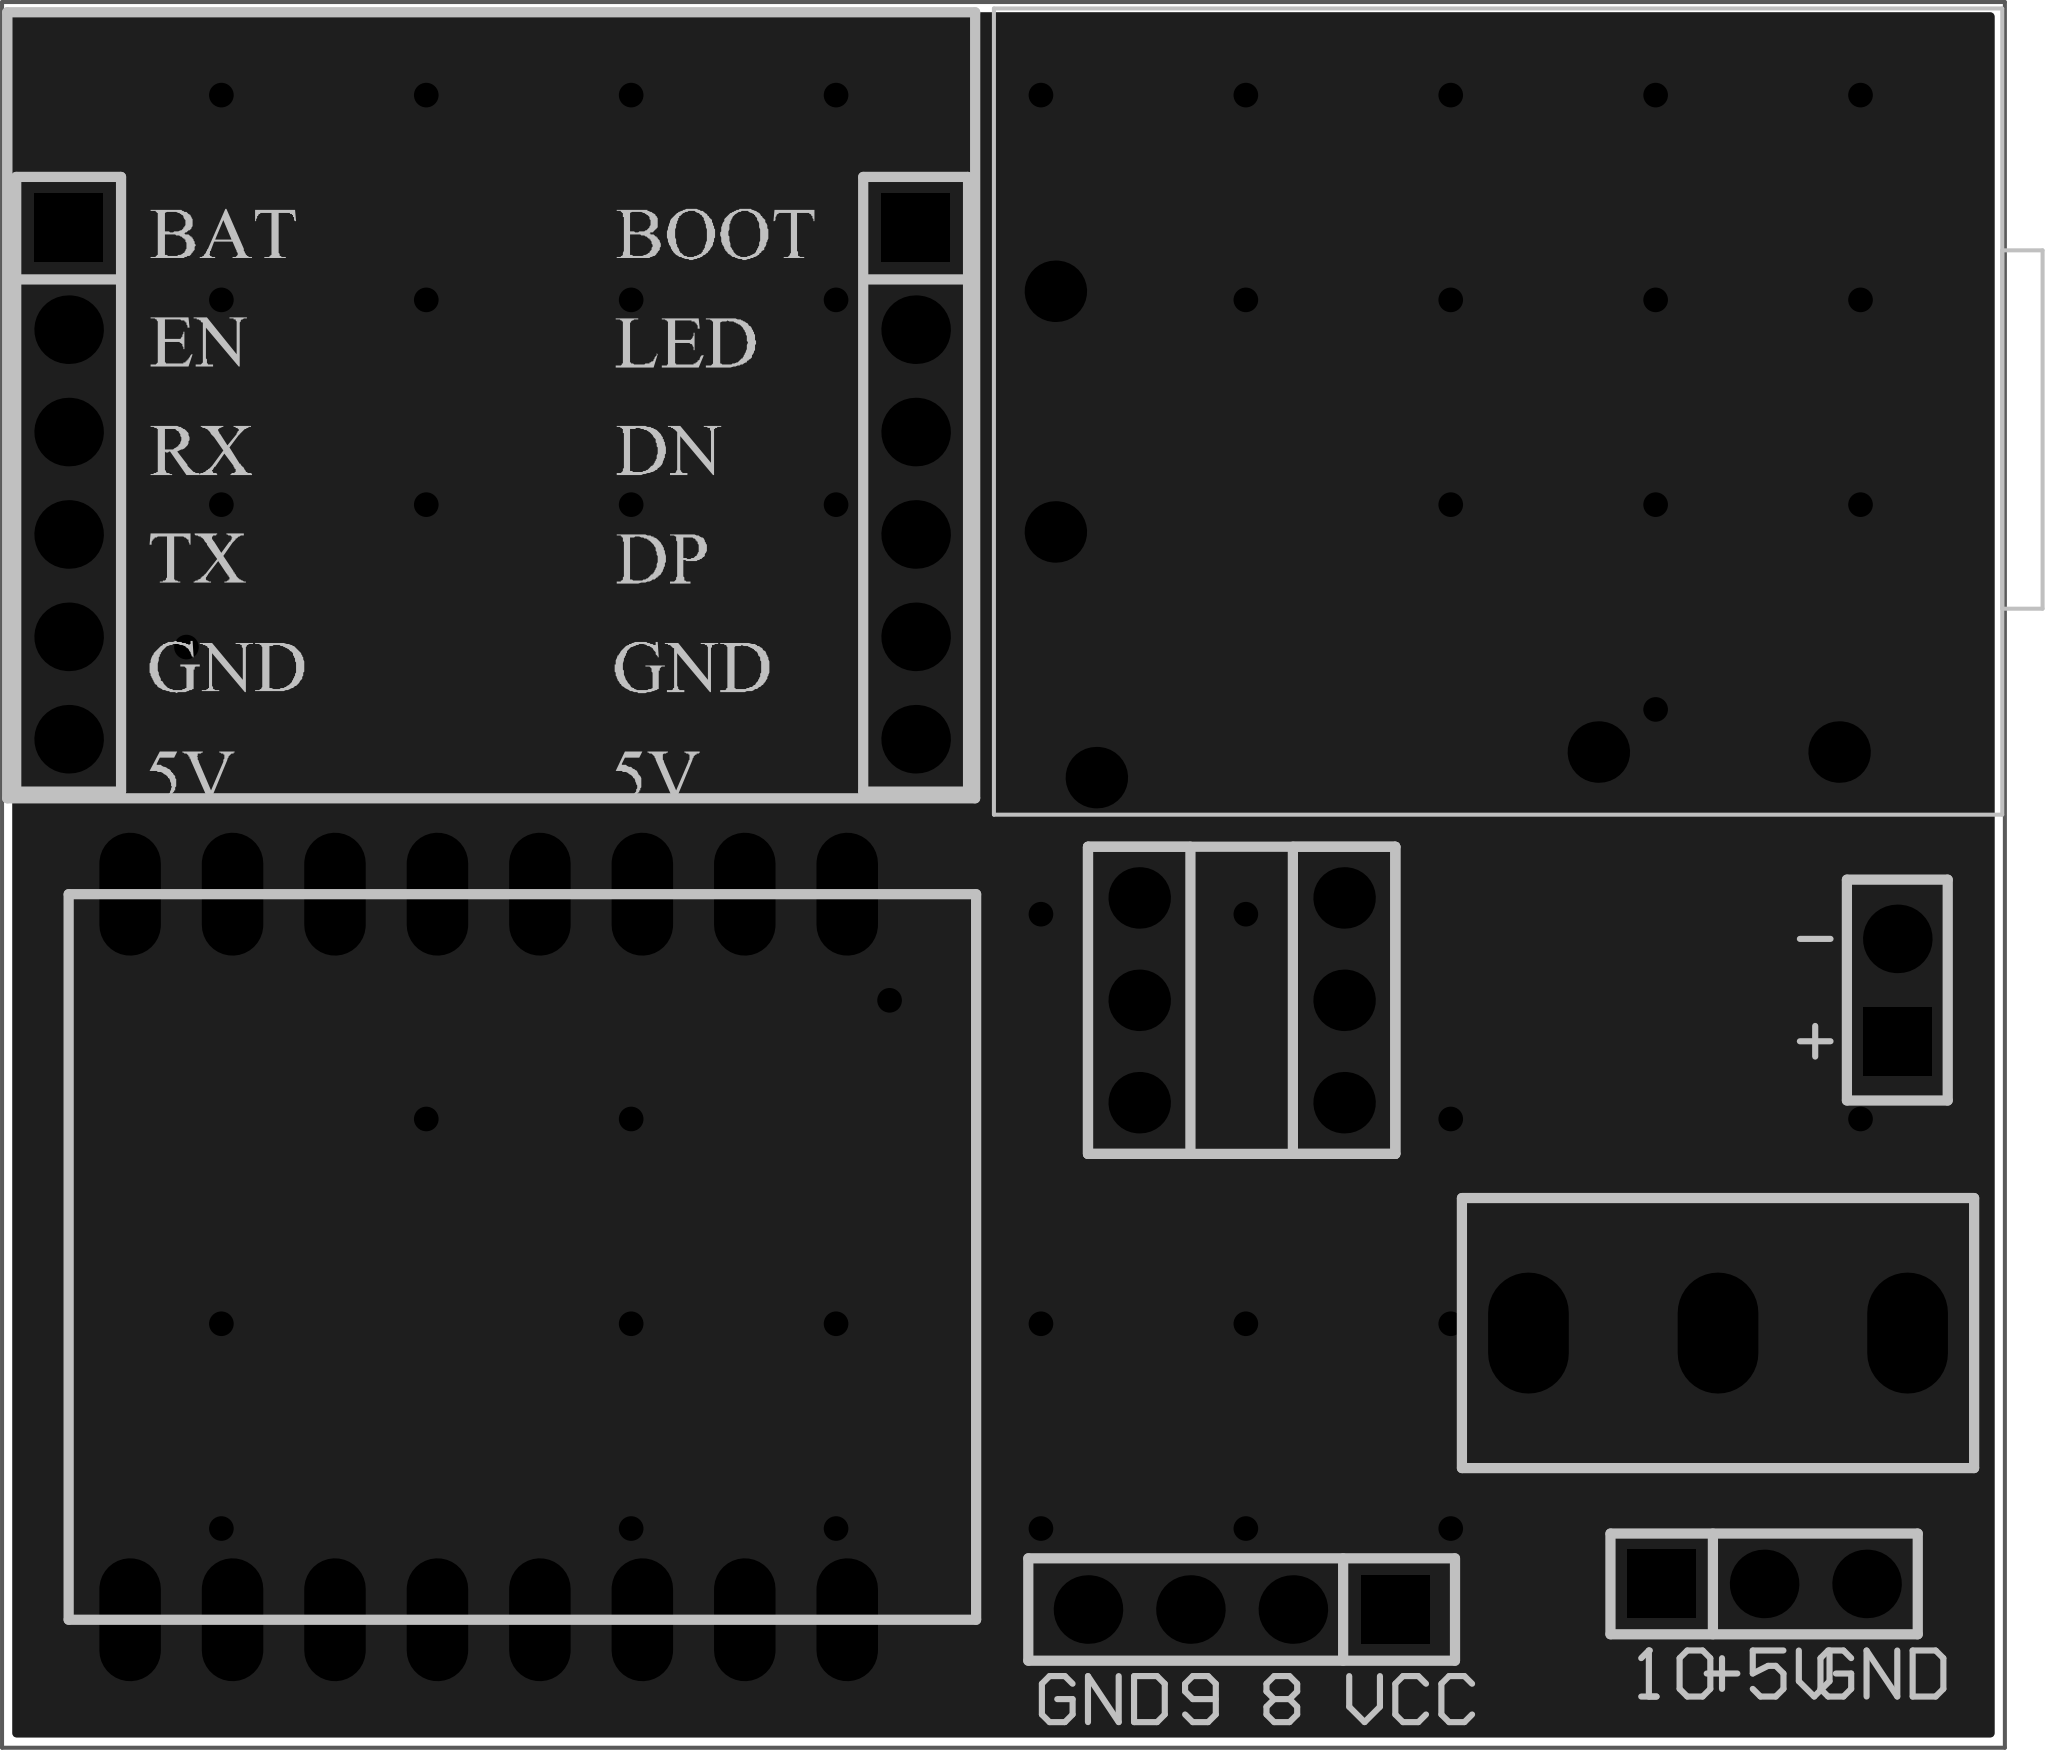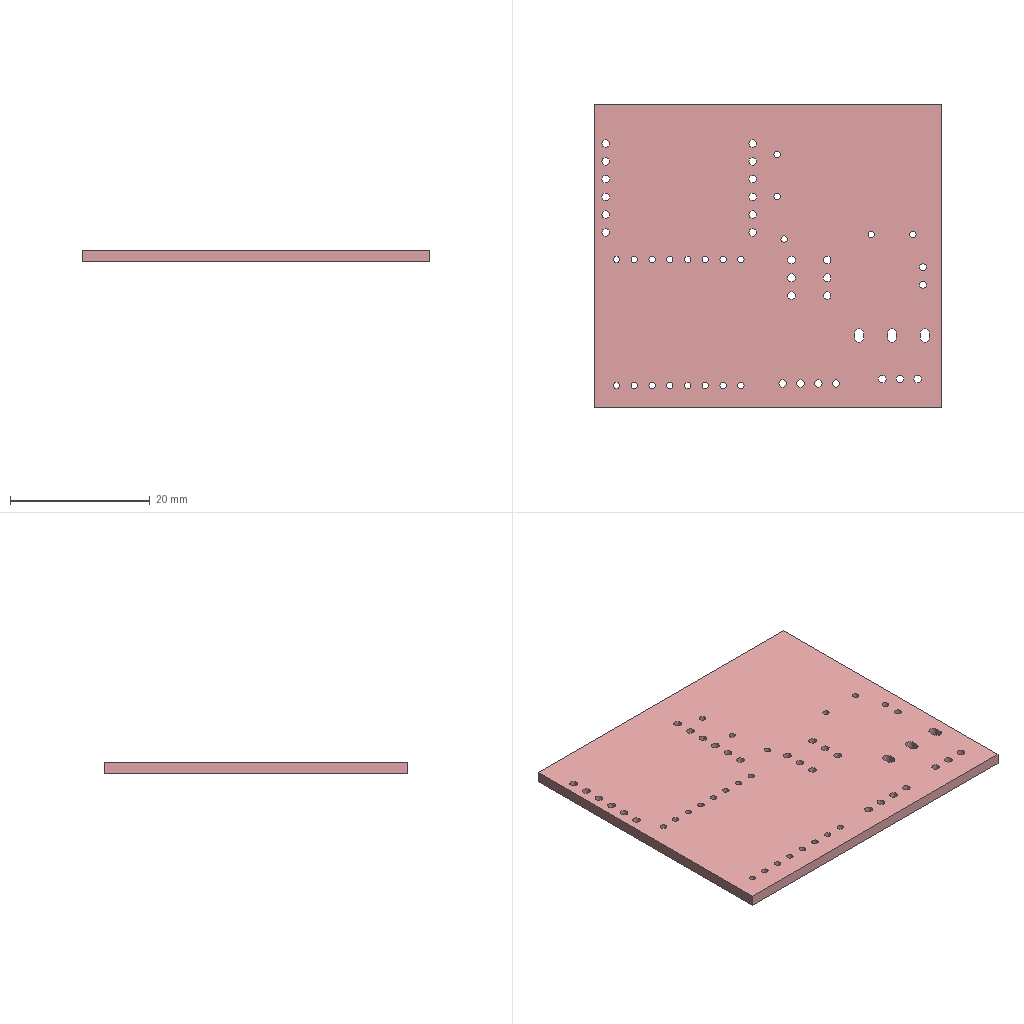Circuit board layout | Altium Designer | box 49.7 x 43.3 x 1.6 mm
Layer stack:
# Altium Designer layer stack of  (unit mm; dielectric type: 0 none, 1 core, 2 prepreg, 3 surface material)
index,name,kind,layer,copper_thickness_mm,dielectric_type,dielectric_thickness_mm,dielectric_material,dielectric_constant
0,Top Paste Mask Layer,other,,,,,,
1,Top Silkscreen Layer,other,,,,,,
2,Top Solder Mask Layer,dielectric,,,3,0.01,,3.3
3,Top Layer,copper,Top Layer,0.035,,,,
4,Dielectric1,dielectric,,,3,1.51,FR4,4.5
5,Bottom Layer,copper,Bottom Layer,0.035,,,,
6,Bottom Solder Mask Layer,dielectric,,,3,0.01,,3.3
7,Bottom Silkscreen Layer,other,,,,,,
8,Bottom Paste Mask Layer,other,,,,,,
# drill layer pairs: low layer,high layer
drill_pair,Top Layer,Bottom Layer
Part placement:
Designator,Comment,Layer,Footprint,Center-X(mm),Center-Y(mm),Rotation
H1,,TopLayer,HDR-TH_3P-P2.54-V-M,161.036,111.506,0
H2,,TopLayer,HDR-TH_2P-P2.54-V-F,164.338,126.238,90
H9,,TopLayer,HDR-TH_4P-P2.54-V-F,148.082,110.871,180
S1,SS-12D10L5,TopLayer,SS-12D10L5,159.893,117.729,0
U3,,TopLayer,【封装Supermini】,129.413,119.617,90
U4,,TopLayer,ML307C-GC核心板,129.499,138.811,0
U5,,TopLayer,5V2A充放电一体模块,153.179,137.541,90
U6,INMP441,TopLayer,INMP441,148.082,125.984,0
Pad and via stacks:
# Altium Designer via and pad stacks of  (unit mm). Each distinct definition once, with the count of objects using it.
# via: kind,start_layer,end_layer,hole_mm,diameter_mm,mode(0 simple;1 top-mid-bottom;2 full stack),diameter_per_layer,count,example_net
# pad: kind,layer,hole_mm,hole_type(0 round;1 square;2 slot),plating,top_size,top_shape(1 round;2 rect;3 octagon;9 rounded rect),mid_size,bottom_size,mode,footprint,size_per_layer,count,example
pad,Multi-Layer,1.1,0,plated,1.7x1.7,2,1.7x1.7,1.7x1.7,0,HDR-TH_3P-P2.54-V-M,,1,H1.1
pad,Multi-Layer,1.1,0,plated,1.7x1.7,1,1.7x1.7,1.7x1.7,0,HDR-TH_3P-P2.54-V-M,,2,H1.2
pad,Multi-Layer,1,0,plated,1.7x1.7,2,1.7x1.7,1.7x1.7,0,HDR-TH_2P-P2.54-V-F,,1,H2.1
pad,Multi-Layer,1,0,plated,1.7x1.7,1,1.7x1.7,1.7x1.7,0,HDR-TH_2P-P2.54-V-F,,1,H2.2
pad,Multi-Layer,1.1,0,plated,1.7x1.7,2,1.7x1.7,1.7x1.7,0,HDR-TH_4P-P2.54-V-F,,1,H9.1
pad,Multi-Layer,1.1,0,plated,1.7x1.7,1,1.7x1.7,1.7x1.7,0,HDR-TH_4P-P2.54-V-F,,3,H9.2
pad,Multi-Layer,1.3,2,plated,2x3,1,2x3,2x3,0,SS-12D10L5,,3,S1.1
pad,Multi-Layer,0.9144,0,plated,1.524x3.048,1,1.524x3.048,1.524x3.048,0,\u00A1\u00BE\u00B7\u00E2\u00D7\u00B0Supermini\u00A1\u00BF,,16,U3.1
pad,Multi-Layer,1.1,0,plated,1.7x1.7,2,1.7x1.7,1.7x1.7,0,ML307C-GC\u00BA\u00CB\u00D0\u00C4\u00B0\u00E5,,2,U4.1
pad,Multi-Layer,1.1,0,plated,1.7x1.7,1,1.7x1.7,1.7x1.7,0,ML307C-GC\u00BA\u00CB\u00D0\u00C4\u00B0\u00E5,,10,U4.2
pad,Multi-Layer,0.9144,0,plated,1.524x1.524,1,1.524x1.524,1.524x1.524,0,5V2A\u00B3\u00E4\u00B7\u00C5\u00B5\u00E7\u00D2\u00BB\u00CC\u00E5\u00C4\u00A3\u00BF\u00E9,,5,U5.3
pad,Multi-Layer,1.1,0,plated,1.524x1.524,1,1.524x1.524,1.524x1.524,0,INMP441,,6,U6.1
via,Top Layer,Bottom Layer,0.3048,0.61,0,,45,VCC
Copper pours:
name,layer,net,type(0 solid;1 hatched;2 none)
Top Layer-GND,Top Layer,GND,0
Bottom Layer-GND,Bottom Layer,GND,0
Design rules, without the lines most boards share:
# Altium Designer design rules of  (exported by Altium Designer, unit mm)
# columns: name | kind | enabled | priority | scope1 | scope2 | descriptor | typed fields (field=value)
Copper_copperRegion_copperThickness1oz | 0 | disabled | 4 | All | All | Clearance Constraint (Gap=5.984mil) (Disabled)(All),(All) | gap=0.152
Copper_copperRegion_copperThickness1oz_1 | 63 | disabled | 4 | All | All | Board Clearance Constraint (Gap=0mil) (Disabled)(All) |
Copper_copperRegion_Copper_copperRegion | 0 | disabled | 5 | All | All | Clearance Constraint (Gap=5.984mil) (Disabled)(All),(All) | gap=0.152
Copper_copperRegion_Copper_copperRegion_1 | 63 | disabled | 5 | All | All | Board Clearance Constraint (Gap=0mil) (Disabled)(All) |
copperThickness1oz | 0 | enabled | 6 | All | All | Clearance Constraint (Gap=5.984mil) (All),(All) | gap=0.152
copperThickness1oz_1 | 63 | enabled | 6 | All | All | Board Clearance Constraint (Gap=0mil) (All) |
copperThickness1oz_2 | 2 | enabled | 2 | All | All | Width Constraint (Min=30mil) (Max=100mil) (Preferred=30mil) (All) |
copperRegion_copperThickness1oz | 20 | enabled | 1 | (InNet('GND')) | All | Polygon Connect Rule(Relief Connect )(Conductor Width=10mil) (Relief Angle=90 Angle) (Entries=4) (Air Gap Width=10mil) ((InNet('GND'))),(All) | connect_style(0=relief,1=direct,2=none)=0 relief_conductor_width=0.254 relief_entries=4
copperRegion_Copper_copperRegion | 20 | disabled | 2 | All | All | Polygon Connect Rule(Relief Connect )(Conductor Width=10mil) (Relief Angle=90 Angle) (Entries=4) (Air Gap Width=10mil) (Disabled)(All),(All) | connect_style(0=relief,1=direct,2=none)=0 relief_conductor_width=0.254 relief_entries=4
copperRegion | 20 | enabled | 3 | All | All | Polygon Connect Rule(Relief Connect )(Conductor Width=10mil) (Relief Angle=90 Angle) (Entries=4) (Air Gap Width=10mil) (All),(All) | connect_style(0=relief,1=direct,2=none)=0 relief_conductor_width=0.254 relief_entries=4